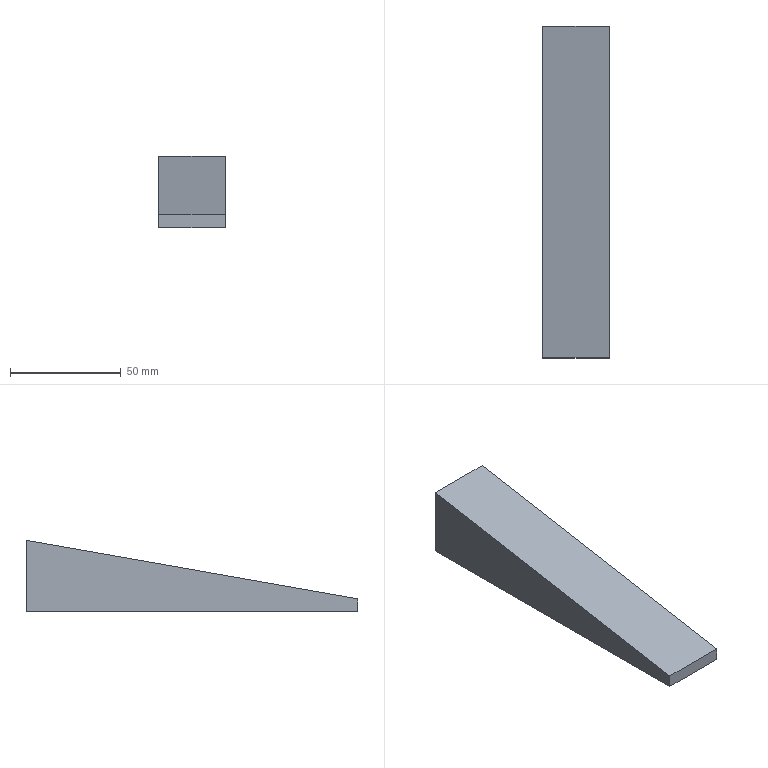Part | NX | features solid 2 | 1 solid | 6 faces | box 30 x 150 x 32.275 mm | volume 85726 mm3 | plane 6
STEP:
#1=CARTESIAN_POINT('',(380.,-450.,-24.174));
#2=VERTEX_POINT('',#1);
#3=CARTESIAN_POINT('',(380.,-300.,2.275));
#4=VERTEX_POINT('',#3);
#5=CARTESIAN_POINT('',(380.,-607.32,-51.914));
#6=DIRECTION('',(0.,0.9848,0.1736));
#7=VECTOR('',#6,1000.);
#8=LINE('',#5,#7);
#9=EDGE_CURVE('',#2,#4,#8,.T.);
#10=ORIENTED_EDGE('',*,*,#9,.T.);
#11=CARTESIAN_POINT('',(350.,-300.,2.275));
#12=VERTEX_POINT('',#11);
#13=CARTESIAN_POINT('',(380.,-300.,2.275));
#14=DIRECTION('',(-1.,0.,0.));
#15=VECTOR('',#14,1000.);
#16=LINE('',#13,#15);
#17=EDGE_CURVE('',#4,#12,#16,.T.);
#18=ORIENTED_EDGE('',*,*,#17,.T.);
#19=CARTESIAN_POINT('',(350.,-450.,-24.174));
#20=VERTEX_POINT('',#19);
#21=CARTESIAN_POINT('',(350.,-607.32,-51.914));
#22=DIRECTION('',(0.,0.9848,0.1736));
#23=VECTOR('',#22,1000.);
#24=LINE('',#21,#23);
#25=EDGE_CURVE('',#20,#12,#24,.T.);
#26=ORIENTED_EDGE('',*,*,#25,.F.);
#27=CARTESIAN_POINT('',(670.,-450.,-24.174));
#28=DIRECTION('',(-1.,0.,0.));
#29=VECTOR('',#28,1000.);
#30=LINE('',#27,#29);
#31=EDGE_CURVE('',#2,#20,#30,.T.);
#32=ORIENTED_EDGE('',*,*,#31,.F.);
#33=EDGE_LOOP('',(#10,#18,#26,#32));
#34=FACE_BOUND('',#33,.T.);
#35=CARTESIAN_POINT('',(340.,-301.969,1.927));
#36=DIRECTION('',(0.,-0.1736,0.9848));
#37=DIRECTION('',(0.,-0.9848,-0.1736));
#38=AXIS2_PLACEMENT_3D('',#35,#36,#37);
#39=PLANE('',#38);
#40=ADVANCED_FACE('',(#34),#39,.T.);
#41=CARTESIAN_POINT('',(380.,-450.,-30.));
#42=VERTEX_POINT('',#41);
#43=CARTESIAN_POINT('',(380.,-450.,20.));
#44=DIRECTION('',(0.,0.,-1.));
#45=VECTOR('',#44,1000.);
#46=LINE('',#43,#45);
#47=EDGE_CURVE('',#2,#42,#46,.T.);
#48=ORIENTED_EDGE('',*,*,#47,.T.);
#49=CARTESIAN_POINT('',(380.,-300.,-30.));
#50=VERTEX_POINT('',#49);
#51=CARTESIAN_POINT('',(380.,-620.,-30.));
#52=DIRECTION('',(0.,1.,0.));
#53=VECTOR('',#52,1000.);
#54=LINE('',#51,#53);
#55=EDGE_CURVE('',#42,#50,#54,.T.);
#56=ORIENTED_EDGE('',*,*,#55,.T.);
#57=CARTESIAN_POINT('',(380.,-300.,20.));
#58=DIRECTION('',(0.,0.,-1.));
#59=VECTOR('',#58,1000.);
#60=LINE('',#57,#59);
#61=EDGE_CURVE('',#4,#50,#60,.T.);
#62=ORIENTED_EDGE('',*,*,#61,.F.);
#63=ORIENTED_EDGE('',*,*,#9,.F.);
#64=EDGE_LOOP('',(#48,#56,#62,#63));
#65=FACE_BOUND('',#64,.T.);
#66=CARTESIAN_POINT('',(380.,-620.,20.));
#67=DIRECTION('',(1.,0.,0.));
#68=DIRECTION('',(0.,0.,1.));
#69=AXIS2_PLACEMENT_3D('',#66,#67,#68);
#70=PLANE('',#69);
#71=ADVANCED_FACE('',(#65),#70,.T.);
#72=ORIENTED_EDGE('',*,*,#31,.T.);
#73=CARTESIAN_POINT('',(350.,-450.,-30.));
#74=VERTEX_POINT('',#73);
#75=CARTESIAN_POINT('',(350.,-450.,20.));
#76=DIRECTION('',(0.,0.,-1.));
#77=VECTOR('',#76,1000.);
#78=LINE('',#75,#77);
#79=EDGE_CURVE('',#20,#74,#78,.T.);
#80=ORIENTED_EDGE('',*,*,#79,.T.);
#81=CARTESIAN_POINT('',(670.,-450.,-30.));
#82=DIRECTION('',(-1.,0.,0.));
#83=VECTOR('',#82,1000.);
#84=LINE('',#81,#83);
#85=EDGE_CURVE('',#42,#74,#84,.T.);
#86=ORIENTED_EDGE('',*,*,#85,.F.);
#87=ORIENTED_EDGE('',*,*,#47,.F.);
#88=EDGE_LOOP('',(#72,#80,#86,#87));
#89=FACE_BOUND('',#88,.T.);
#90=CARTESIAN_POINT('',(670.,-450.,20.));
#91=DIRECTION('',(0.,1.,0.));
#92=DIRECTION('',(0.,0.,1.));
#93=AXIS2_PLACEMENT_3D('',#90,#91,#92);
#94=PLANE('',#93);
#95=ADVANCED_FACE('',(#89),#94,.F.);
#96=ORIENTED_EDGE('',*,*,#25,.T.);
#97=CARTESIAN_POINT('',(350.,-300.,-30.));
#98=VERTEX_POINT('',#97);
#99=CARTESIAN_POINT('',(350.,-300.,20.));
#100=DIRECTION('',(0.,0.,-1.));
#101=VECTOR('',#100,1000.);
#102=LINE('',#99,#101);
#103=EDGE_CURVE('',#12,#98,#102,.T.);
#104=ORIENTED_EDGE('',*,*,#103,.T.);
#105=CARTESIAN_POINT('',(350.,-620.,-30.));
#106=DIRECTION('',(0.,1.,0.));
#107=VECTOR('',#106,1000.);
#108=LINE('',#105,#107);
#109=EDGE_CURVE('',#74,#98,#108,.T.);
#110=ORIENTED_EDGE('',*,*,#109,.F.);
#111=ORIENTED_EDGE('',*,*,#79,.F.);
#112=EDGE_LOOP('',(#96,#104,#110,#111));
#113=FACE_BOUND('',#112,.T.);
#114=CARTESIAN_POINT('',(350.,-620.,20.));
#115=DIRECTION('',(1.,0.,0.));
#116=DIRECTION('',(0.,0.,1.));
#117=AXIS2_PLACEMENT_3D('',#114,#115,#116);
#118=PLANE('',#117);
#119=ADVANCED_FACE('',(#113),#118,.F.);
#120=ORIENTED_EDGE('',*,*,#61,.T.);
#121=CARTESIAN_POINT('',(380.,-300.,-30.));
#122=DIRECTION('',(-1.,0.,0.));
#123=VECTOR('',#122,1000.);
#124=LINE('',#121,#123);
#125=EDGE_CURVE('',#50,#98,#124,.T.);
#126=ORIENTED_EDGE('',*,*,#125,.T.);
#127=ORIENTED_EDGE('',*,*,#103,.F.);
#128=ORIENTED_EDGE('',*,*,#17,.F.);
#129=EDGE_LOOP('',(#120,#126,#127,#128));
#130=FACE_BOUND('',#129,.T.);
#131=CARTESIAN_POINT('',(380.,-300.,20.));
#132=DIRECTION('',(0.,1.,0.));
#133=DIRECTION('',(0.,0.,1.));
#134=AXIS2_PLACEMENT_3D('',#131,#132,#133);
#135=PLANE('',#134);
#136=ADVANCED_FACE('',(#130),#135,.T.);
#137=ORIENTED_EDGE('',*,*,#55,.F.);
#138=ORIENTED_EDGE('',*,*,#85,.T.);
#139=ORIENTED_EDGE('',*,*,#109,.T.);
#140=ORIENTED_EDGE('',*,*,#125,.F.);
#141=EDGE_LOOP('',(#137,#138,#139,#140));
#142=FACE_BOUND('',#141,.T.);
#143=CARTESIAN_POINT('',(445.,-540.,-30.));
#144=DIRECTION('',(0.,0.,1.));
#145=DIRECTION('',(-1.,0.,0.));
#146=AXIS2_PLACEMENT_3D('',#143,#144,#145);
#147=PLANE('',#146);
#148=ADVANCED_FACE('',(#142),#147,.F.);
#149=CLOSED_SHELL('',(#40,#71,#95,#119,#136,#148));
#150=MANIFOLD_SOLID_BREP('',#149);
#151=(LENGTH_UNIT()NAMED_UNIT(*)SI_UNIT(.MILLI.,.METRE.));
#152=UNCERTAINTY_MEASURE_WITH_UNIT(LENGTH_MEASURE(0.00001),#151,'','');
#153=(NAMED_UNIT(*)PLANE_ANGLE_UNIT()SI_UNIT($,.RADIAN.));
#154=(NAMED_UNIT(*)SI_UNIT($,.STERADIAN.)SOLID_ANGLE_UNIT());
#155=(GEOMETRIC_REPRESENTATION_CONTEXT(3)GLOBAL_UNCERTAINTY_ASSIGNED_CONTEXT((#152))GLOBAL_UNIT_ASSIGNED_CONTEXT((#151,#153,#154))REPRESENTATION_CONTEXT('',''));
#156=ADVANCED_BREP_SHAPE_REPRESENTATION('',(#150),#155);